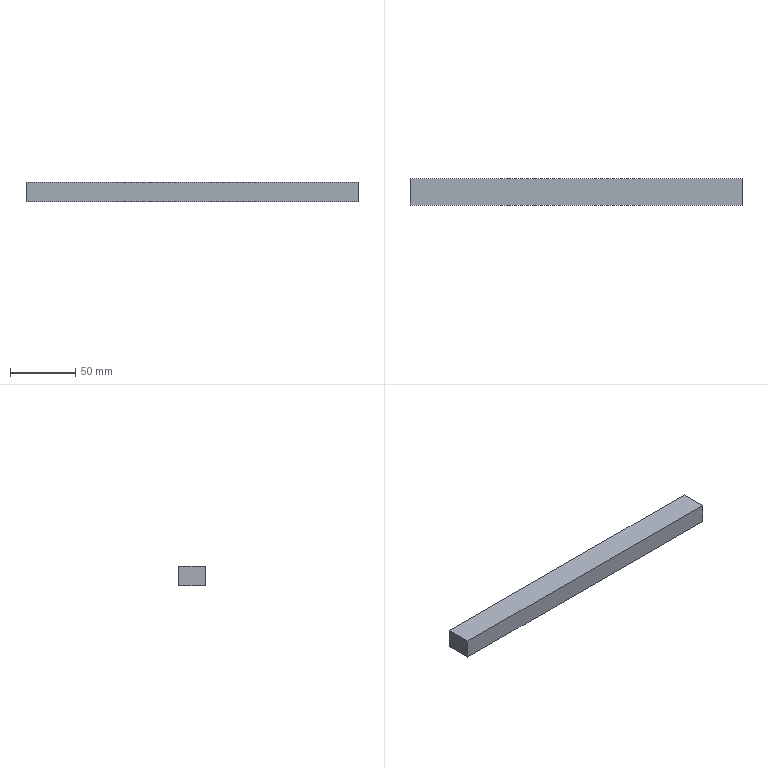Part | NX | features DATUM_CSYS 2, EXTRUDE 1, SKETCH 1 | 1 solid | 6 faces | box 255 x 20 x 15 mm | volume 76500 mm3 | plane 6
STEP:
#1=CARTESIAN_POINT('',(-127.5,10.,0.));
#2=VERTEX_POINT('',#1);
#3=CARTESIAN_POINT('',(-127.5,-10.,0.));
#4=VERTEX_POINT('',#3);
#5=CARTESIAN_POINT('',(-127.5,10.,0.));
#6=DIRECTION('',(0.,-1.,0.));
#7=VECTOR('',#6,1000.);
#8=LINE('',#5,#7);
#9=EDGE_CURVE('',#2,#4,#8,.T.);
#10=ORIENTED_EDGE('',*,*,#9,.T.);
#11=CARTESIAN_POINT('',(-127.5,-10.,15.));
#12=VERTEX_POINT('',#11);
#13=CARTESIAN_POINT('',(-127.5,-10.,15.));
#14=DIRECTION('',(0.,0.,-1.));
#15=VECTOR('',#14,1000.);
#16=LINE('',#13,#15);
#17=EDGE_CURVE('',#12,#4,#16,.T.);
#18=ORIENTED_EDGE('',*,*,#17,.F.);
#19=CARTESIAN_POINT('',(-127.5,10.,15.));
#20=VERTEX_POINT('',#19);
#21=CARTESIAN_POINT('',(-127.5,10.,15.));
#22=DIRECTION('',(0.,-1.,0.));
#23=VECTOR('',#22,1000.);
#24=LINE('',#21,#23);
#25=EDGE_CURVE('',#20,#12,#24,.T.);
#26=ORIENTED_EDGE('',*,*,#25,.F.);
#27=CARTESIAN_POINT('',(-127.5,10.,15.));
#28=DIRECTION('',(0.,0.,-1.));
#29=VECTOR('',#28,1000.);
#30=LINE('',#27,#29);
#31=EDGE_CURVE('',#20,#2,#30,.T.);
#32=ORIENTED_EDGE('',*,*,#31,.T.);
#33=EDGE_LOOP('',(#10,#18,#26,#32));
#34=FACE_BOUND('',#33,.T.);
#35=CARTESIAN_POINT('',(-127.5,10.,15.));
#36=DIRECTION('',(1.,0.,0.));
#37=DIRECTION('',(0.,1.,0.));
#38=AXIS2_PLACEMENT_3D('',#35,#36,#37);
#39=PLANE('',#38);
#40=ADVANCED_FACE('',(#34),#39,.F.);
#41=CARTESIAN_POINT('',(127.5,-10.,0.));
#42=VERTEX_POINT('',#41);
#43=CARTESIAN_POINT('',(-127.5,-10.,0.));
#44=DIRECTION('',(1.,0.,0.));
#45=VECTOR('',#44,1000.);
#46=LINE('',#43,#45);
#47=EDGE_CURVE('',#4,#42,#46,.T.);
#48=ORIENTED_EDGE('',*,*,#47,.T.);
#49=CARTESIAN_POINT('',(127.5,-10.,15.));
#50=VERTEX_POINT('',#49);
#51=CARTESIAN_POINT('',(127.5,-10.,15.));
#52=DIRECTION('',(0.,0.,-1.));
#53=VECTOR('',#52,1000.);
#54=LINE('',#51,#53);
#55=EDGE_CURVE('',#50,#42,#54,.T.);
#56=ORIENTED_EDGE('',*,*,#55,.F.);
#57=CARTESIAN_POINT('',(-127.5,-10.,15.));
#58=DIRECTION('',(1.,0.,0.));
#59=VECTOR('',#58,1000.);
#60=LINE('',#57,#59);
#61=EDGE_CURVE('',#12,#50,#60,.T.);
#62=ORIENTED_EDGE('',*,*,#61,.F.);
#63=ORIENTED_EDGE('',*,*,#17,.T.);
#64=EDGE_LOOP('',(#48,#56,#62,#63));
#65=FACE_BOUND('',#64,.T.);
#66=CARTESIAN_POINT('',(-127.5,-10.,15.));
#67=DIRECTION('',(0.,1.,0.));
#68=DIRECTION('',(0.,0.,1.));
#69=AXIS2_PLACEMENT_3D('',#66,#67,#68);
#70=PLANE('',#69);
#71=ADVANCED_FACE('',(#65),#70,.F.);
#72=CARTESIAN_POINT('',(127.5,10.,0.));
#73=VERTEX_POINT('',#72);
#74=CARTESIAN_POINT('',(127.5,-10.,0.));
#75=DIRECTION('',(0.,1.,0.));
#76=VECTOR('',#75,1000.);
#77=LINE('',#74,#76);
#78=EDGE_CURVE('',#42,#73,#77,.T.);
#79=ORIENTED_EDGE('',*,*,#78,.T.);
#80=CARTESIAN_POINT('',(127.5,10.,15.));
#81=VERTEX_POINT('',#80);
#82=CARTESIAN_POINT('',(127.5,10.,15.));
#83=DIRECTION('',(0.,0.,-1.));
#84=VECTOR('',#83,1000.);
#85=LINE('',#82,#84);
#86=EDGE_CURVE('',#81,#73,#85,.T.);
#87=ORIENTED_EDGE('',*,*,#86,.F.);
#88=CARTESIAN_POINT('',(127.5,-10.,15.));
#89=DIRECTION('',(0.,1.,0.));
#90=VECTOR('',#89,1000.);
#91=LINE('',#88,#90);
#92=EDGE_CURVE('',#50,#81,#91,.T.);
#93=ORIENTED_EDGE('',*,*,#92,.F.);
#94=ORIENTED_EDGE('',*,*,#55,.T.);
#95=EDGE_LOOP('',(#79,#87,#93,#94));
#96=FACE_BOUND('',#95,.T.);
#97=CARTESIAN_POINT('',(127.5,-10.,15.));
#98=DIRECTION('',(-1.,0.,0.));
#99=DIRECTION('',(0.,-1.,0.));
#100=AXIS2_PLACEMENT_3D('',#97,#98,#99);
#101=PLANE('',#100);
#102=ADVANCED_FACE('',(#96),#101,.F.);
#103=CARTESIAN_POINT('',(127.5,10.,0.));
#104=DIRECTION('',(-1.,0.,0.));
#105=VECTOR('',#104,1000.);
#106=LINE('',#103,#105);
#107=EDGE_CURVE('',#73,#2,#106,.T.);
#108=ORIENTED_EDGE('',*,*,#107,.T.);
#109=ORIENTED_EDGE('',*,*,#31,.F.);
#110=CARTESIAN_POINT('',(127.5,10.,15.));
#111=DIRECTION('',(-1.,0.,0.));
#112=VECTOR('',#111,1000.);
#113=LINE('',#110,#112);
#114=EDGE_CURVE('',#81,#20,#113,.T.);
#115=ORIENTED_EDGE('',*,*,#114,.F.);
#116=ORIENTED_EDGE('',*,*,#86,.T.);
#117=EDGE_LOOP('',(#108,#109,#115,#116));
#118=FACE_BOUND('',#117,.T.);
#119=CARTESIAN_POINT('',(127.5,10.,15.));
#120=DIRECTION('',(0.,-1.,0.));
#121=DIRECTION('',(0.,0.,-1.));
#122=AXIS2_PLACEMENT_3D('',#119,#120,#121);
#123=PLANE('',#122);
#124=ADVANCED_FACE('',(#118),#123,.F.);
#125=ORIENTED_EDGE('',*,*,#25,.T.);
#126=ORIENTED_EDGE('',*,*,#61,.T.);
#127=ORIENTED_EDGE('',*,*,#92,.T.);
#128=ORIENTED_EDGE('',*,*,#114,.T.);
#129=EDGE_LOOP('',(#125,#126,#127,#128));
#130=FACE_BOUND('',#129,.T.);
#131=CARTESIAN_POINT('',(0.,0.,15.));
#132=DIRECTION('',(0.,0.,1.));
#133=DIRECTION('',(1.,0.,0.));
#134=AXIS2_PLACEMENT_3D('',#131,#132,#133);
#135=PLANE('',#134);
#136=ADVANCED_FACE('',(#130),#135,.T.);
#137=ORIENTED_EDGE('',*,*,#9,.F.);
#138=ORIENTED_EDGE('',*,*,#107,.F.);
#139=ORIENTED_EDGE('',*,*,#78,.F.);
#140=ORIENTED_EDGE('',*,*,#47,.F.);
#141=EDGE_LOOP('',(#137,#138,#139,#140));
#142=FACE_BOUND('',#141,.T.);
#143=CARTESIAN_POINT('',(0.,0.,0.));
#144=DIRECTION('',(0.,0.,1.));
#145=DIRECTION('',(1.,0.,0.));
#146=AXIS2_PLACEMENT_3D('',#143,#144,#145);
#147=PLANE('',#146);
#148=ADVANCED_FACE('',(#142),#147,.F.);
#149=CLOSED_SHELL('',(#40,#71,#102,#124,#136,#148));
#150=MANIFOLD_SOLID_BREP('',#149);
#151=(LENGTH_UNIT()NAMED_UNIT(*)SI_UNIT(.MILLI.,.METRE.));
#152=UNCERTAINTY_MEASURE_WITH_UNIT(LENGTH_MEASURE(0.00001),#151,'','');
#153=(NAMED_UNIT(*)PLANE_ANGLE_UNIT()SI_UNIT($,.RADIAN.));
#154=(NAMED_UNIT(*)SI_UNIT($,.STERADIAN.)SOLID_ANGLE_UNIT());
#155=(GEOMETRIC_REPRESENTATION_CONTEXT(3)GLOBAL_UNCERTAINTY_ASSIGNED_CONTEXT((#152))GLOBAL_UNIT_ASSIGNED_CONTEXT((#151,#153,#154))REPRESENTATION_CONTEXT('',''));
#156=ADVANCED_BREP_SHAPE_REPRESENTATION('',(#150),#155);